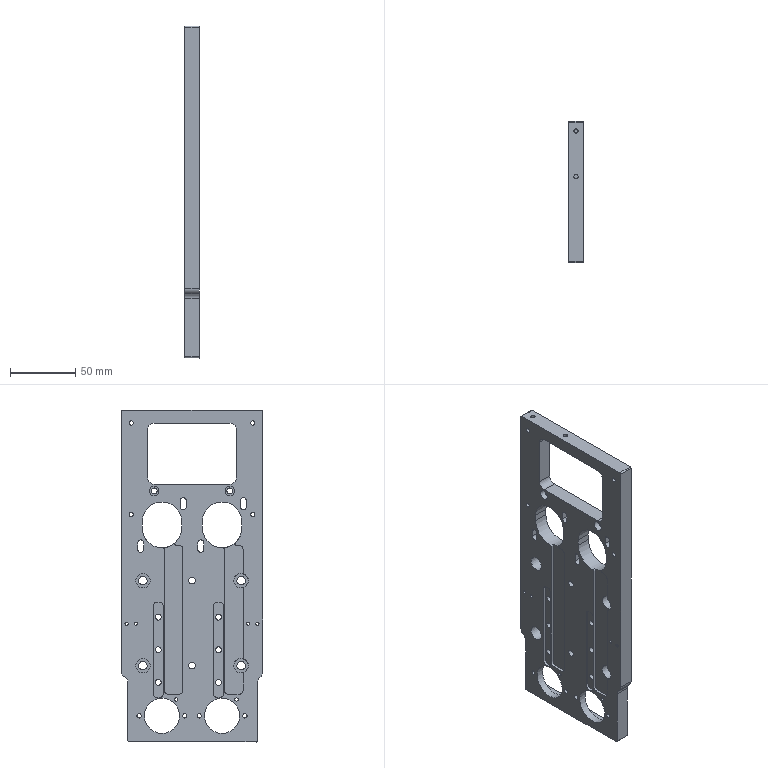CAM job | NX | 3+2 milling, drilling | part box 11 x 108 x 253.9 mm | stock box 15 x 110 x 258.9 mm
Tools:
number,name,description,diameter,corner_radius,flute_length,length,flutes
4,D4,平底铣刀-粗,4.0,0.0,25.0,75.0,2
6,D6,平底铣刀-粗,6.0,0.0,25.0,75.0,2
9,D10,平底铣刀-粗,10.0,0.0,35.0,75.0,2
18,D3-J,平底铣刀-精,3.0,0.0,50.0,75.0,2
17,D4-J,平底铣刀-精,4.0,0.0,50.0,75.0,2
7,D6-J,平底铣刀-精,6.0,0.0,25.0,75.0,2
10,D10-J,平底铣刀-精,10.0,0.0,35.0,75.0,2
1,D80R0.8飞刀,圆鼻刀-粗,80.0,0.8,50.0,75.0,2
1,D80R0.8飞刀-J,圆鼻刀-精,80.0,0.8,50.0,75.0,2
2,D6倒角刀,倒角刀,6.0,0.0,3.0,25.0,2
20,M3X0.5,丝锥,2.5,0.0,35.0,50.0,2
21,M4X0.7,丝锥,3.3,0.0,35.0,50.0,2
12,ZT2.5,钻头,2.5,0.0,35.0,50.0,2
11,ZT4.5,钻头,4.5,0.0,35.0,50.0,2
23,ZT6.5,钻头,6.5,0.0,35.0,50.0,2
22,ZT10,钻头,10.0,0.0,35.0,50.0,2
13,钻头3.3,Twist Drill 3.3 mm,3.3,0.0,35.0,35.008,2
19,ZT4.9,Drilling Tool,4.9,0.0,35.0,50.0,2
Operations:
program,operation,operation_type,tool,method,geometry_group,spindle_rpm,surface_speed,feed_per_tooth,feed_cut,feed_plunge,cut_length_mm,path_length_mm,cut_time_min,machine_time_min
B,底壁铣飞面开粗_COPY,VolumeBased25DMillingOperation,D80R0.8飞刀,分层开粗-切深K-步距G,W-B,2800.0,703.696,0.5357,3000.0,100.0,5937.232,6339.469,1.979,2.019
B,底壁铣飞面精光_COPY,VolumeBased25DMillingOperation,D80R0.8飞刀-J,侧刃精光-切深K-步距G,W-B,4000.0,1005.28,0.125,1000.0,100.0,741.567,777.567,0.7416,0.7452
B,底壁铣分层开粗-中_COPY,VolumeBased25DMillingOperation,D10,分层开粗-切深K-步距G,W-B,8000.0,251.32,0.25,4000.0,100.0,5094.234,5292.181,1.274,1.293
B,铣沉头_1,CylinderMilling,D4,METHOD,W-B,8000.0,100.531,0.1125,1800.0,100.0,964.066,1396.266,0.5356,0.5788
B,铣孔_1,CylinderMilling,D4,METHOD,W-B,8000.0,100.531,0.0375,600.0,100.0,92.705,553.705,0.1545,0.2006
B,C0.3封闭铣廓倒角6X45L_COPY,PlanarMilling,D6倒角刀,爬面_倒角-切深0-步距G,W-B,7000.0,131.0,0.1071,1500.0,100.0,457.473,663.086,0.305,0.3255
B,钻倒角_3,Operation,D6倒角刀,METHOD,W-B,8000.0,150.796,0.0625,1000.0,0.0,28.5,298.369,0.0285,0.0555
B,钻倒角_4,Operation,D6倒角刀,METHOD,W-B,8000.0,150.796,0.0625,1000.0,0.0,36.4,535.111,0.0364,0.0863
B,钻倒角_5,Operation,D6倒角刀,METHOD,W-B,8000.0,150.796,0.0625,1000.0,0.0,11.1,123.278,0.0111,0.0223
B,铣倒角_1,PlanarMilling,D6倒角刀,METHOD,W-B,8000.0,150.796,0.075,1200.0,100.0,25.104,173.708,0.0209,0.0358
B,铣倒角_4,PlanarMilling,D6倒角刀,METHOD,W-B,8000.0,150.796,0.075,1200.0,100.0,80.763,455.142,0.0673,0.1047
B,平面去毛刺6X45L_COPY_1,SurfaceContour,D6倒角刀,爬面_倒角-切深0-步距G,W-B,6500.0,122.519,0.1154,1500.0,100.0,1952.21,3794.278,1.302,1.486
B,等高光顺清角D4参考10_COPY,ZLevelMilling,D4-J,分层精光-切深K-步距G,W-B,8000.0,100.528,0.0625,1000.0,100.0,554.286,805.549,0.5543,0.5794
B,底壁铣精光底面-中_COPY,VolumeBased25DMillingOperation,D6-J,精光步距切深关,W-B,8000.0,150.792,0.0625,1000.0,100.0,859.754,894.481,0.8598,0.8632
B,底壁铣精光侧面-中-选底面_COPY,VolumeBased25DMillingOperation,D6-J,侧刃精光-切深K-步距G,W-B,8000.0,150.792,0.0625,1000.0,100.0,217.391,253.618,0.2174,0.221
A,顶面,FaceMilling,D80R0.8飞刀,侧刃精光-切深K-步距G,W-A,4000.0,1005.31,0.125,1000.0,100.0,1109.7,1145.7,1.11,1.113
A,外形粗_2,VolumeBased25DMillingOperation,D10,METHOD,W-A,8000.0,251.327,0.3125,5000.0,80.0,11972.614,12022.314,2.394,2.4
A,底壁粗_1,VolumeBased25DMillingOperation,D10,METHOD,W-A,6000.0,113.0,0.2083,3500.0,100.0,1048.212,1205.163,0.2995,0.3152
A,底壁粗_2,VolumeBased25DMillingOperation,D10,METHOD,W-A,6000.0,113.0,0.2083,3500.0,100.0,1022.386,1179.337,0.2921,0.3078
A,框开粗_1,VolumeBased25DMillingOperation,D10,METHOD,W-A,6000.0,188.0,0.25,4000.0,80.0,8036.52,8330.958,2.009,2.039
A,腰槽粗,VolumeBased25DMillingOperation,D6,METHOD,W-A,6000.0,113.0,0.2083,2500.0,100.0,3005.565,3132.567,1.202,1.215
A,通腰槽粗_1,VolumeBased25DMillingOperation,D4,METHOD,W-A,6000.0,75.398,0.1,1200.0,100.0,3518.376,3843.156,2.932,2.965
A,打点-深0.8,Operation,D6倒角刀,NONE,W-A,8000.0,150.796,0.0312,500.0,90.0,54.0,922.659,0.108,0.1949
A,通孔-M3螺纹底孔,Operation,ZT2.5,NONE,W-A,3000.0,23.562,0.05,300.0,90.0,95.906,421.455,0.3197,0.3522
A,通孔-M4螺纹底孔,Operation,钻头3.3,NONE,W-A,3000.0,31.102,0.05,300.0,90.0,104.74,653.587,0.3491,0.404
A,盲平孔-M4螺纹底孔,Operation,钻头3.3,NONE,W-A,3000.0,31.102,0.0167,100.0,90.0,18.0,76.0,0.18,0.1858
A,通孔-5-6,Operation,ZT4.5,NONE,W-A,3000.0,42.411,0.025,150.0,90.0,65.112,321.314,0.4341,0.4597
A,沉头孔-钻孔0段,Operation,ZT4.5,NONE,W-A,2800.0,39.584,0.0179,100.0,90.0,30.704,160.416,0.307,0.32
A,通孔-精孔6.0预钻,Operation,ZT4.9,NONE,W-A,2500.0,38.484,0.05,250.0,90.0,32.829,171.666,0.1313,0.1452
A,沉头孔-钻孔0段_2,Operation,ZT6.5,NONE,W-A,1200.0,24.504,0.0625,150.0,90.0,63.811,375.644,0.4254,0.4566
A,通孔-8-10,Operation,ZT10,NONE,W-A,1800.0,152.681,0.0417,150.0,90.0,30.0,147.011,0.2,0.2117
A,底壁铣螺旋开粗-中_COPY,VolumeBased25DMillingOperation,D10,分层开粗-切深K-步距G,W-A,8000.0,251.327,0.1875,3000.0,100.0,1313.803,1456.87,0.4379,0.4522
A,铣孔开粗D6_1,CylinderMilling,D6,NONE,W-A,8000.0,150.796,0.075,1200.0,100.0,1116.457,1511.457,0.9304,0.9699
A,铣孔开粗D4_2,CylinderMilling,D4,NONE,W-A,8000.0,100.531,0.075,1200.0,100.0,376.822,522.822,0.314,0.3286
A,铣孔精光D6_1,CylinderMilling,D6-J,精光步距切深关,W-A,8000.0,150.796,0.0312,500.0,100.0,199.561,596.561,0.3991,0.4388
A,清角D4,ZLevelMilling,D6-J,METHOD,W-A,6000.0,75.0,0.25,2500.0,80.0,610.927,1023.974,0.245,0.2863
A,底精_1,VolumeBased25DMillingOperation,D6-J,METHOD,W-A,6000.0,113.0,0.2083,1200.0,100.0,486.221,528.221,0.4052,0.4094
A,底精_2,VolumeBased25DMillingOperation,D6-J,METHOD,W-A,6000.0,113.0,0.2083,1200.0,100.0,460.347,503.347,0.3836,0.3879
A,平面去毛刺6X45L_COPY,SurfaceContour,D6倒角刀,爬面_倒角-切深0-步距G,W-A,6500.0,122.519,0.1154,1500.0,100.0,2475.24,4736.026,1.65,1.876
A,钻倒角_1,Operation,D6倒角刀,METHOD,W-A,8000.0,150.796,0.0312,500.0,0.0,28.5,297.947,0.057,0.0839
A,钻倒角_2,Operation,D6倒角刀,METHOD,W-A,8000.0,150.796,0.0312,500.0,0.0,41.6,613.081,0.0832,0.1403
A,铣倒角_2,PlanarMilling,D6倒角刀,METHOD,W-A,8000.0,150.796,0.0312,500.0,100.0,37.057,184.076,0.0741,0.0888
A,铣倒角_3,PlanarMilling,D6倒角刀,NONE,W-A,8000.0,150.796,0.0312,500.0,100.0,64.794,194.646,0.1296,0.1426
A,铣倒角_5,PlanarMilling,D6倒角刀,METHOD,W-A,8000.0,150.796,0.05,800.0,100.0,181.699,315.699,0.2271,0.2405
A,通孔-攻牙M3,Operation,M3X0.5,METHOD,W-A,800.0,6.283,0.0003,0.5,90.0,79.4,388.442,158.8,158.831
A,通孔-攻牙M4,Operation,M4X0.7,METHOD,W-A,600.0,6.22,0.0006,0.7,90.0,83.8,611.707,119.714,119.767
A,盲平孔-攻牙M4,Operation,M4X0.7,METHOD,W-A,800.0,8.294,0.0004,0.7,90.0,15.0,70.0,21.429,21.434
A,底壁铣螺旋精光-中_COPY,VolumeBased25DMillingOperation,D3-J,螺旋精光-切深K-步距G,W-A,6000.0,56.549,0.025,300.0,100.0,217.794,382.767,0.726,0.7425
A,铣孔精光D4_1,CylinderMilling,D4-J,精光步距切深关,W-A,8000.0,100.531,0.0312,500.0,100.0,57.015,203.015,0.114,0.1286
A,腰槽精_3,VolumeBased25DMillingOperation,D4-J,METHOD,W-A,6000.0,113.0,0.0417,500.0,100.0,166.343,611.126,0.3327,0.3772
A,框精_1,VolumeBased25DMillingOperation,D6-J,METHOD,W-A,6000.0,113.0,0.0833,1000.0,100.0,390.033,736.421,0.39,0.4247
A,底侧精_3,VolumeBased25DMillingOperation,D6-J,METHOD,W-A,6000.0,113.0,0.2083,1200.0,100.0,265.135,408.57,0.2209,0.2353
A,腰槽精,VolumeBased25DMillingOperation,D6-J,METHOD,W-A,6000.0,113.0,0.0667,600.0,100.0,278.897,411.969,0.4648,0.4781
A,底侧精_4,VolumeBased25DMillingOperation,D6-J,METHOD,W-A,6000.0,113.0,0.2083,1200.0,100.0,252.482,295.472,0.2104,0.2147
A,外形半精_2,VolumeBased25DMillingOperation,D10-J,METHOD,W-A,8000.0,251.327,0.0625,1000.0,100.0,752.554,813.954,0.7526,0.7587
A,底壁铣精光侧面-中_COPY,VolumeBased25DMillingOperation,D10-J,侧刃精光-切深K-步距G,W-A,8000.0,251.327,0.0375,600.0,100.0,124.864,232.975,0.2081,0.2189